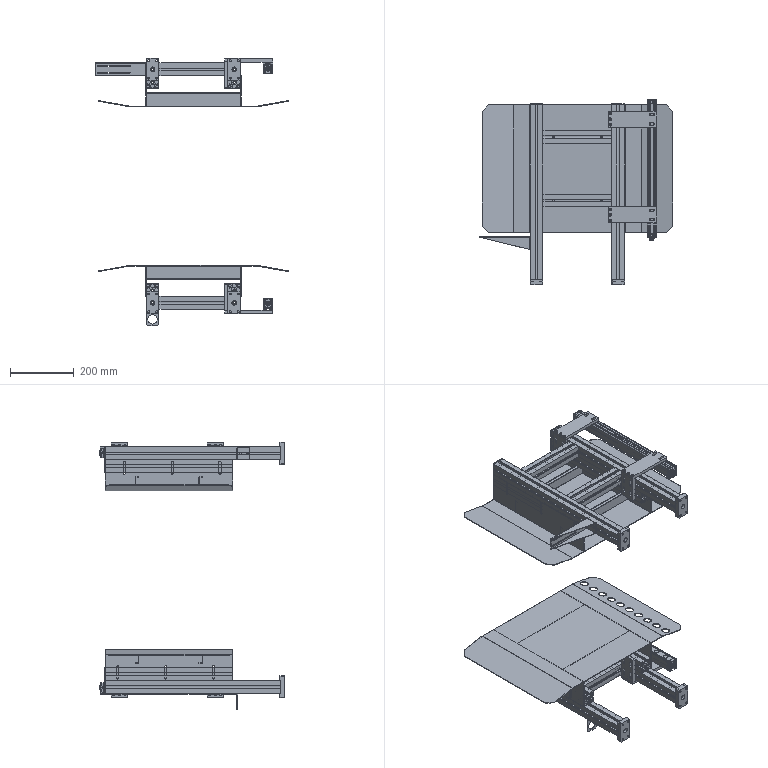Part | NX | 70 solids | 3025 faces | volume 6067366 mm3 | plane 1762 | cylinder 873 | spline 238 | cone 152 | commonest cylinder face diameters 0.4 x220 2 x96 0.8 x60 8 x60 7 x48 20 x48